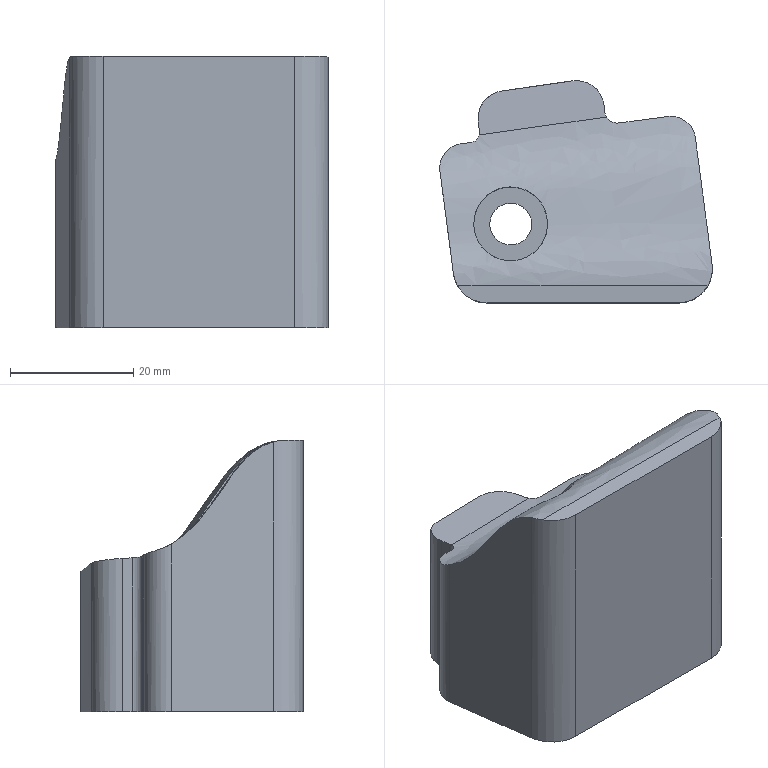Part | STEP file | gslz 2016.10.28-13_id1506_x_t | 1 solid | 23 faces | box 44.234 x 36.078 x 44 mm | volume 40757 mm3 | plane 11 | cylinder 10 | other 1 | spline 1 | commonest cylinder face diameters 8 x2 9 x2 11 x2 3 x1 4 x1 6.8 x1